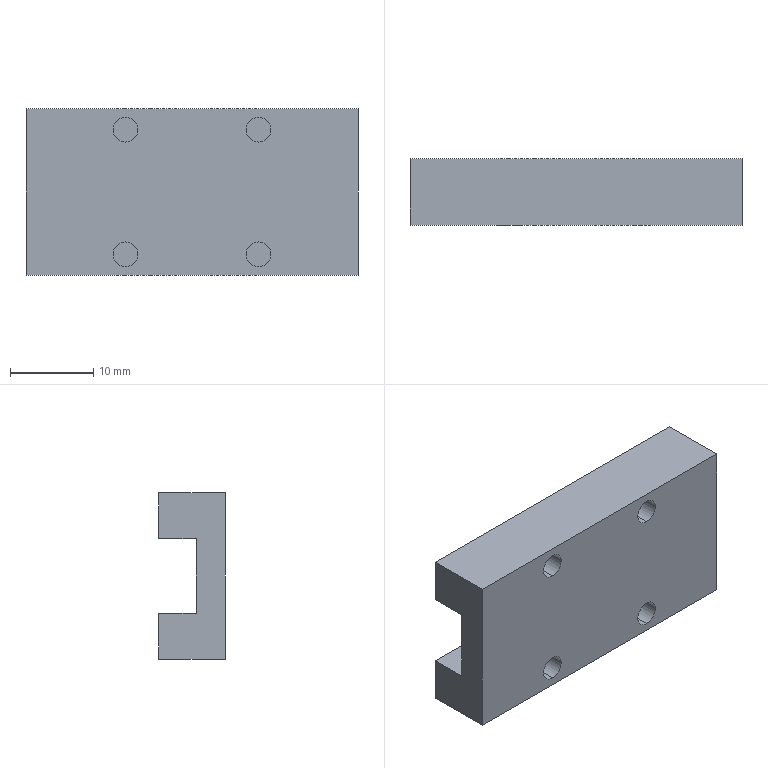Part | SolidWorks | features BaseBody 1 | 1 solid | 22 faces | box 39.9 x 8 x 20 mm | volume 4655 mm3 | plane 14 | cylinder 8 | commonest cylinder face diameters 3 x8
STEP:
#1=CARTESIAN_POINT('',(-8.,4.,9.));
#2=VERTEX_POINT('',#1);
#3=CARTESIAN_POINT('',(-8.,4.,6.));
#4=VERTEX_POINT('',#3);
#5=CARTESIAN_POINT('',(-8.,4.,7.5));
#6=DIRECTION('',(0.,-1.,0.));
#7=DIRECTION('',(0.,0.,-1.));
#8=AXIS2_PLACEMENT_3D('',#5,#6,#7);
#9=CIRCLE('',#8,1.5);
#10=EDGE_CURVE('',#2,#4,#9,.T.);
#11=ORIENTED_EDGE('',*,*,#10,.F.);
#12=CARTESIAN_POINT('',(-8.,0.,9.));
#13=VERTEX_POINT('',#12);
#14=CARTESIAN_POINT('',(-8.,4.,9.));
#15=DIRECTION('',(0.,-1.,0.));
#16=VECTOR('',#15,1000.);
#17=LINE('',#14,#16);
#18=EDGE_CURVE('',#2,#13,#17,.T.);
#19=ORIENTED_EDGE('',*,*,#18,.T.);
#20=CARTESIAN_POINT('',(-8.,0.,6.));
#21=VERTEX_POINT('',#20);
#22=CARTESIAN_POINT('',(-8.,0.,7.5));
#23=DIRECTION('',(0.,1.,0.));
#24=DIRECTION('',(0.,0.,-1.));
#25=AXIS2_PLACEMENT_3D('',#22,#23,#24);
#26=CIRCLE('',#25,1.5);
#27=EDGE_CURVE('',#21,#13,#26,.T.);
#28=ORIENTED_EDGE('',*,*,#27,.F.);
#29=CARTESIAN_POINT('',(-8.,4.,6.));
#30=DIRECTION('',(0.,-1.,0.));
#31=VECTOR('',#30,1000.);
#32=LINE('',#29,#31);
#33=EDGE_CURVE('',#4,#21,#32,.T.);
#34=ORIENTED_EDGE('',*,*,#33,.F.);
#35=EDGE_LOOP('',(#11,#19,#28,#34));
#36=FACE_OUTER_BOUND('',#35,.T.);
#37=CARTESIAN_POINT('',(-8.,4.,7.5));
#38=DIRECTION('',(0.,-1.,0.));
#39=DIRECTION('',(0.,0.,-1.));
#40=AXIS2_PLACEMENT_3D('',#37,#38,#39);
#41=CYLINDRICAL_SURFACE('',#40,1.5);
#42=ADVANCED_FACE('',(#36),#41,.F.);
#43=CARTESIAN_POINT('',(8.,4.,9.));
#44=VERTEX_POINT('',#43);
#45=CARTESIAN_POINT('',(8.,4.,6.));
#46=VERTEX_POINT('',#45);
#47=CARTESIAN_POINT('',(8.,4.,7.5));
#48=DIRECTION('',(0.,-1.,0.));
#49=DIRECTION('',(0.,0.,-1.));
#50=AXIS2_PLACEMENT_3D('',#47,#48,#49);
#51=CIRCLE('',#50,1.5);
#52=EDGE_CURVE('',#44,#46,#51,.T.);
#53=ORIENTED_EDGE('',*,*,#52,.F.);
#54=CARTESIAN_POINT('',(8.,0.,9.));
#55=VERTEX_POINT('',#54);
#56=CARTESIAN_POINT('',(8.,4.,9.));
#57=DIRECTION('',(0.,-1.,0.));
#58=VECTOR('',#57,1000.);
#59=LINE('',#56,#58);
#60=EDGE_CURVE('',#44,#55,#59,.T.);
#61=ORIENTED_EDGE('',*,*,#60,.T.);
#62=CARTESIAN_POINT('',(8.,0.,6.));
#63=VERTEX_POINT('',#62);
#64=CARTESIAN_POINT('',(8.,0.,7.5));
#65=DIRECTION('',(0.,1.,0.));
#66=DIRECTION('',(0.,0.,-1.));
#67=AXIS2_PLACEMENT_3D('',#64,#65,#66);
#68=CIRCLE('',#67,1.5);
#69=EDGE_CURVE('',#63,#55,#68,.T.);
#70=ORIENTED_EDGE('',*,*,#69,.F.);
#71=CARTESIAN_POINT('',(8.,4.,6.));
#72=DIRECTION('',(0.,-1.,0.));
#73=VECTOR('',#72,1000.);
#74=LINE('',#71,#73);
#75=EDGE_CURVE('',#46,#63,#74,.T.);
#76=ORIENTED_EDGE('',*,*,#75,.F.);
#77=EDGE_LOOP('',(#53,#61,#70,#76));
#78=FACE_OUTER_BOUND('',#77,.T.);
#79=CARTESIAN_POINT('',(8.,4.,7.5));
#80=DIRECTION('',(0.,-1.,0.));
#81=DIRECTION('',(0.,0.,-1.));
#82=AXIS2_PLACEMENT_3D('',#79,#80,#81);
#83=CYLINDRICAL_SURFACE('',#82,1.5);
#84=ADVANCED_FACE('',(#78),#83,.F.);
#85=CARTESIAN_POINT('',(8.,4.,-6.));
#86=VERTEX_POINT('',#85);
#87=CARTESIAN_POINT('',(8.,4.,-9.));
#88=VERTEX_POINT('',#87);
#89=CARTESIAN_POINT('',(8.,4.,-7.5));
#90=DIRECTION('',(0.,-1.,0.));
#91=DIRECTION('',(0.,0.,-1.));
#92=AXIS2_PLACEMENT_3D('',#89,#90,#91);
#93=CIRCLE('',#92,1.5);
#94=EDGE_CURVE('',#86,#88,#93,.T.);
#95=ORIENTED_EDGE('',*,*,#94,.F.);
#96=CARTESIAN_POINT('',(8.,0.,-6.));
#97=VERTEX_POINT('',#96);
#98=CARTESIAN_POINT('',(8.,4.,-6.));
#99=DIRECTION('',(0.,-1.,0.));
#100=VECTOR('',#99,1000.);
#101=LINE('',#98,#100);
#102=EDGE_CURVE('',#86,#97,#101,.T.);
#103=ORIENTED_EDGE('',*,*,#102,.T.);
#104=CARTESIAN_POINT('',(8.,0.,-9.));
#105=VERTEX_POINT('',#104);
#106=CARTESIAN_POINT('',(8.,0.,-7.5));
#107=DIRECTION('',(0.,1.,0.));
#108=DIRECTION('',(0.,0.,-1.));
#109=AXIS2_PLACEMENT_3D('',#106,#107,#108);
#110=CIRCLE('',#109,1.5);
#111=EDGE_CURVE('',#105,#97,#110,.T.);
#112=ORIENTED_EDGE('',*,*,#111,.F.);
#113=CARTESIAN_POINT('',(8.,4.,-9.));
#114=DIRECTION('',(0.,-1.,0.));
#115=VECTOR('',#114,1000.);
#116=LINE('',#113,#115);
#117=EDGE_CURVE('',#88,#105,#116,.T.);
#118=ORIENTED_EDGE('',*,*,#117,.F.);
#119=EDGE_LOOP('',(#95,#103,#112,#118));
#120=FACE_OUTER_BOUND('',#119,.T.);
#121=CARTESIAN_POINT('',(8.,4.,-7.5));
#122=DIRECTION('',(0.,-1.,0.));
#123=DIRECTION('',(0.,0.,-1.));
#124=AXIS2_PLACEMENT_3D('',#121,#122,#123);
#125=CYLINDRICAL_SURFACE('',#124,1.5);
#126=ADVANCED_FACE('',(#120),#125,.F.);
#127=CARTESIAN_POINT('',(-8.,4.,-6.));
#128=VERTEX_POINT('',#127);
#129=CARTESIAN_POINT('',(-8.,4.,-9.));
#130=VERTEX_POINT('',#129);
#131=CARTESIAN_POINT('',(-8.,4.,-7.5));
#132=DIRECTION('',(0.,-1.,0.));
#133=DIRECTION('',(0.,0.,-1.));
#134=AXIS2_PLACEMENT_3D('',#131,#132,#133);
#135=CIRCLE('',#134,1.5);
#136=EDGE_CURVE('',#128,#130,#135,.T.);
#137=ORIENTED_EDGE('',*,*,#136,.F.);
#138=CARTESIAN_POINT('',(-8.,0.,-6.));
#139=VERTEX_POINT('',#138);
#140=CARTESIAN_POINT('',(-8.,4.,-6.));
#141=DIRECTION('',(0.,-1.,0.));
#142=VECTOR('',#141,1000.);
#143=LINE('',#140,#142);
#144=EDGE_CURVE('',#128,#139,#143,.T.);
#145=ORIENTED_EDGE('',*,*,#144,.T.);
#146=CARTESIAN_POINT('',(-8.,0.,-9.));
#147=VERTEX_POINT('',#146);
#148=CARTESIAN_POINT('',(-8.,0.,-7.5));
#149=DIRECTION('',(0.,1.,0.));
#150=DIRECTION('',(0.,0.,-1.));
#151=AXIS2_PLACEMENT_3D('',#148,#149,#150);
#152=CIRCLE('',#151,1.5);
#153=EDGE_CURVE('',#147,#139,#152,.T.);
#154=ORIENTED_EDGE('',*,*,#153,.F.);
#155=CARTESIAN_POINT('',(-8.,4.,-9.));
#156=DIRECTION('',(0.,-1.,0.));
#157=VECTOR('',#156,1000.);
#158=LINE('',#155,#157);
#159=EDGE_CURVE('',#130,#147,#158,.T.);
#160=ORIENTED_EDGE('',*,*,#159,.F.);
#161=EDGE_LOOP('',(#137,#145,#154,#160));
#162=FACE_OUTER_BOUND('',#161,.T.);
#163=CARTESIAN_POINT('',(-8.,4.,-7.5));
#164=DIRECTION('',(0.,-1.,0.));
#165=DIRECTION('',(0.,0.,-1.));
#166=AXIS2_PLACEMENT_3D('',#163,#164,#165);
#167=CYLINDRICAL_SURFACE('',#166,1.5);
#168=ADVANCED_FACE('',(#162),#167,.F.);
#169=CARTESIAN_POINT('',(-19.95,0.,-10.));
#170=VERTEX_POINT('',#169);
#171=CARTESIAN_POINT('',(19.95,0.,-10.));
#172=VERTEX_POINT('',#171);
#173=CARTESIAN_POINT('',(0.,0.,-10.));
#174=DIRECTION('',(1.,0.,0.));
#175=VECTOR('',#174,1000.);
#176=LINE('',#173,#175);
#177=EDGE_CURVE('',#170,#172,#176,.T.);
#178=ORIENTED_EDGE('',*,*,#177,.T.);
#179=CARTESIAN_POINT('',(19.95,0.,10.));
#180=VERTEX_POINT('',#179);
#181=CARTESIAN_POINT('',(19.95,0.,0.));
#182=DIRECTION('',(0.,0.,1.));
#183=VECTOR('',#182,1000.);
#184=LINE('',#181,#183);
#185=EDGE_CURVE('',#172,#180,#184,.T.);
#186=ORIENTED_EDGE('',*,*,#185,.T.);
#187=CARTESIAN_POINT('',(-19.95,0.,10.));
#188=VERTEX_POINT('',#187);
#189=CARTESIAN_POINT('',(0.,0.,10.));
#190=DIRECTION('',(-1.,0.,0.));
#191=VECTOR('',#190,1000.);
#192=LINE('',#189,#191);
#193=EDGE_CURVE('',#180,#188,#192,.T.);
#194=ORIENTED_EDGE('',*,*,#193,.T.);
#195=CARTESIAN_POINT('',(-19.95,0.,0.));
#196=DIRECTION('',(0.,0.,-1.));
#197=VECTOR('',#196,1000.);
#198=LINE('',#195,#197);
#199=EDGE_CURVE('',#188,#170,#198,.T.);
#200=ORIENTED_EDGE('',*,*,#199,.T.);
#201=EDGE_LOOP('',(#178,#186,#194,#200));
#202=FACE_OUTER_BOUND('',#201,.T.);
#203=ORIENTED_EDGE('',*,*,#27,.T.);
#204=CARTESIAN_POINT('',(-8.,0.,7.5));
#205=DIRECTION('',(0.,1.,0.));
#206=DIRECTION('',(0.,0.,-1.));
#207=AXIS2_PLACEMENT_3D('',#204,#205,#206);
#208=CIRCLE('',#207,1.5);
#209=EDGE_CURVE('',#13,#21,#208,.T.);
#210=ORIENTED_EDGE('',*,*,#209,.T.);
#211=EDGE_LOOP('',(#203,#210));
#212=FACE_BOUND('',#211,.T.);
#213=ORIENTED_EDGE('',*,*,#69,.T.);
#214=CARTESIAN_POINT('',(8.,0.,7.5));
#215=DIRECTION('',(0.,1.,0.));
#216=DIRECTION('',(0.,0.,-1.));
#217=AXIS2_PLACEMENT_3D('',#214,#215,#216);
#218=CIRCLE('',#217,1.5);
#219=EDGE_CURVE('',#55,#63,#218,.T.);
#220=ORIENTED_EDGE('',*,*,#219,.T.);
#221=EDGE_LOOP('',(#213,#220));
#222=FACE_BOUND('',#221,.T.);
#223=ORIENTED_EDGE('',*,*,#111,.T.);
#224=CARTESIAN_POINT('',(8.,0.,-7.5));
#225=DIRECTION('',(0.,1.,0.));
#226=DIRECTION('',(0.,0.,-1.));
#227=AXIS2_PLACEMENT_3D('',#224,#225,#226);
#228=CIRCLE('',#227,1.5);
#229=EDGE_CURVE('',#97,#105,#228,.T.);
#230=ORIENTED_EDGE('',*,*,#229,.T.);
#231=EDGE_LOOP('',(#223,#230));
#232=FACE_BOUND('',#231,.T.);
#233=ORIENTED_EDGE('',*,*,#153,.T.);
#234=CARTESIAN_POINT('',(-8.,0.,-7.5));
#235=DIRECTION('',(0.,1.,0.));
#236=DIRECTION('',(0.,0.,-1.));
#237=AXIS2_PLACEMENT_3D('',#234,#235,#236);
#238=CIRCLE('',#237,1.5);
#239=EDGE_CURVE('',#139,#147,#238,.T.);
#240=ORIENTED_EDGE('',*,*,#239,.T.);
#241=EDGE_LOOP('',(#233,#240));
#242=FACE_BOUND('',#241,.T.);
#243=CARTESIAN_POINT('',(0.,0.,0.));
#244=DIRECTION('',(0.,-1.,0.));
#245=DIRECTION('',(0.,0.,-1.));
#246=AXIS2_PLACEMENT_3D('',#243,#244,#245);
#247=PLANE('',#246);
#248=ADVANCED_FACE('',(#202,#212,#222,#232,#242),#247,.T.);
#249=CARTESIAN_POINT('',(19.95,8.,-10.));
#250=VERTEX_POINT('',#249);
#251=CARTESIAN_POINT('',(-19.95,8.,-10.));
#252=VERTEX_POINT('',#251);
#253=CARTESIAN_POINT('',(-19.95,8.,-10.));
#254=DIRECTION('',(-1.,0.,0.));
#255=VECTOR('',#254,1000.);
#256=LINE('',#253,#255);
#257=EDGE_CURVE('',#250,#252,#256,.T.);
#258=ORIENTED_EDGE('',*,*,#257,.F.);
#259=CARTESIAN_POINT('',(19.95,8.,-10.));
#260=DIRECTION('',(0.,-1.,0.));
#261=VECTOR('',#260,1000.);
#262=LINE('',#259,#261);
#263=EDGE_CURVE('',#250,#172,#262,.T.);
#264=ORIENTED_EDGE('',*,*,#263,.T.);
#265=ORIENTED_EDGE('',*,*,#177,.F.);
#266=CARTESIAN_POINT('',(-19.95,8.,-10.));
#267=DIRECTION('',(0.,-1.,0.));
#268=VECTOR('',#267,1000.);
#269=LINE('',#266,#268);
#270=EDGE_CURVE('',#252,#170,#269,.T.);
#271=ORIENTED_EDGE('',*,*,#270,.F.);
#272=EDGE_LOOP('',(#258,#264,#265,#271));
#273=FACE_OUTER_BOUND('',#272,.T.);
#274=CARTESIAN_POINT('',(-19.95,8.,-10.));
#275=DIRECTION('',(0.,0.,1.));
#276=DIRECTION('',(1.,0.,0.));
#277=AXIS2_PLACEMENT_3D('',#274,#275,#276);
#278=PLANE('',#277);
#279=ADVANCED_FACE('',(#273),#278,.F.);
#280=ORIENTED_EDGE('',*,*,#193,.F.);
#281=CARTESIAN_POINT('',(19.95,8.,10.));
#282=VERTEX_POINT('',#281);
#283=CARTESIAN_POINT('',(19.95,8.,10.));
#284=DIRECTION('',(0.,1.,0.));
#285=VECTOR('',#284,1000.);
#286=LINE('',#283,#285);
#287=EDGE_CURVE('',#180,#282,#286,.T.);
#288=ORIENTED_EDGE('',*,*,#287,.T.);
#289=CARTESIAN_POINT('',(-19.95,8.,10.));
#290=VERTEX_POINT('',#289);
#291=CARTESIAN_POINT('',(-19.95,8.,10.));
#292=DIRECTION('',(1.,0.,0.));
#293=VECTOR('',#292,1000.);
#294=LINE('',#291,#293);
#295=EDGE_CURVE('',#290,#282,#294,.T.);
#296=ORIENTED_EDGE('',*,*,#295,.F.);
#297=CARTESIAN_POINT('',(-19.95,8.,10.));
#298=DIRECTION('',(0.,-1.,0.));
#299=VECTOR('',#298,1000.);
#300=LINE('',#297,#299);
#301=EDGE_CURVE('',#290,#188,#300,.T.);
#302=ORIENTED_EDGE('',*,*,#301,.T.);
#303=EDGE_LOOP('',(#280,#288,#296,#302));
#304=FACE_OUTER_BOUND('',#303,.T.);
#305=CARTESIAN_POINT('',(-19.95,8.,10.));
#306=DIRECTION('',(0.,0.,-1.));
#307=DIRECTION('',(-1.,0.,0.));
#308=AXIS2_PLACEMENT_3D('',#305,#306,#307);
#309=PLANE('',#308);
#310=ADVANCED_FACE('',(#304),#309,.F.);
#311=ORIENTED_EDGE('',*,*,#18,.F.);
#312=CARTESIAN_POINT('',(-8.,4.,7.5));
#313=DIRECTION('',(0.,-1.,0.));
#314=DIRECTION('',(0.,0.,-1.));
#315=AXIS2_PLACEMENT_3D('',#312,#313,#314);
#316=CIRCLE('',#315,1.5);
#317=EDGE_CURVE('',#4,#2,#316,.T.);
#318=ORIENTED_EDGE('',*,*,#317,.F.);
#319=ORIENTED_EDGE('',*,*,#33,.T.);
#320=ORIENTED_EDGE('',*,*,#209,.F.);
#321=EDGE_LOOP('',(#311,#318,#319,#320));
#322=FACE_OUTER_BOUND('',#321,.T.);
#323=CARTESIAN_POINT('',(-8.,4.,7.5));
#324=DIRECTION('',(0.,-1.,0.));
#325=DIRECTION('',(0.,0.,-1.));
#326=AXIS2_PLACEMENT_3D('',#323,#324,#325);
#327=CYLINDRICAL_SURFACE('',#326,1.5);
#328=ADVANCED_FACE('',(#322),#327,.F.);
#329=ORIENTED_EDGE('',*,*,#60,.F.);
#330=CARTESIAN_POINT('',(8.,4.,7.5));
#331=DIRECTION('',(0.,-1.,0.));
#332=DIRECTION('',(0.,0.,-1.));
#333=AXIS2_PLACEMENT_3D('',#330,#331,#332);
#334=CIRCLE('',#333,1.5);
#335=EDGE_CURVE('',#46,#44,#334,.T.);
#336=ORIENTED_EDGE('',*,*,#335,.F.);
#337=ORIENTED_EDGE('',*,*,#75,.T.);
#338=ORIENTED_EDGE('',*,*,#219,.F.);
#339=EDGE_LOOP('',(#329,#336,#337,#338));
#340=FACE_OUTER_BOUND('',#339,.T.);
#341=CARTESIAN_POINT('',(8.,4.,7.5));
#342=DIRECTION('',(0.,-1.,0.));
#343=DIRECTION('',(0.,0.,-1.));
#344=AXIS2_PLACEMENT_3D('',#341,#342,#343);
#345=CYLINDRICAL_SURFACE('',#344,1.5);
#346=ADVANCED_FACE('',(#340),#345,.F.);
#347=ORIENTED_EDGE('',*,*,#102,.F.);
#348=CARTESIAN_POINT('',(8.,4.,-7.5));
#349=DIRECTION('',(0.,-1.,0.));
#350=DIRECTION('',(0.,0.,-1.));
#351=AXIS2_PLACEMENT_3D('',#348,#349,#350);
#352=CIRCLE('',#351,1.5);
#353=EDGE_CURVE('',#88,#86,#352,.T.);
#354=ORIENTED_EDGE('',*,*,#353,.F.);
#355=ORIENTED_EDGE('',*,*,#117,.T.);
#356=ORIENTED_EDGE('',*,*,#229,.F.);
#357=EDGE_LOOP('',(#347,#354,#355,#356));
#358=FACE_OUTER_BOUND('',#357,.T.);
#359=CARTESIAN_POINT('',(8.,4.,-7.5));
#360=DIRECTION('',(0.,-1.,0.));
#361=DIRECTION('',(0.,0.,-1.));
#362=AXIS2_PLACEMENT_3D('',#359,#360,#361);
#363=CYLINDRICAL_SURFACE('',#362,1.5);
#364=ADVANCED_FACE('',(#358),#363,.F.);
#365=ORIENTED_EDGE('',*,*,#144,.F.);
#366=CARTESIAN_POINT('',(-8.,4.,-7.5));
#367=DIRECTION('',(0.,-1.,0.));
#368=DIRECTION('',(0.,0.,-1.));
#369=AXIS2_PLACEMENT_3D('',#366,#367,#368);
#370=CIRCLE('',#369,1.5);
#371=EDGE_CURVE('',#130,#128,#370,.T.);
#372=ORIENTED_EDGE('',*,*,#371,.F.);
#373=ORIENTED_EDGE('',*,*,#159,.T.);
#374=ORIENTED_EDGE('',*,*,#239,.F.);
#375=EDGE_LOOP('',(#365,#372,#373,#374));
#376=FACE_OUTER_BOUND('',#375,.T.);
#377=CARTESIAN_POINT('',(-8.,4.,-7.5));
#378=DIRECTION('',(0.,-1.,0.));
#379=DIRECTION('',(0.,0.,-1.));
#380=AXIS2_PLACEMENT_3D('',#377,#378,#379);
#381=CYLINDRICAL_SURFACE('',#380,1.5);
#382=ADVANCED_FACE('',(#376),#381,.F.);
#383=CARTESIAN_POINT('',(19.95,8.,-4.5));
#384=VERTEX_POINT('',#383);
#385=CARTESIAN_POINT('',(-19.95,8.,-4.5));
#386=VERTEX_POINT('',#385);
#387=CARTESIAN_POINT('',(0.,8.,-4.5));
#388=DIRECTION('',(-1.,0.,0.));
#389=VECTOR('',#388,1000.);
#390=LINE('',#387,#389);
#391=EDGE_CURVE('',#384,#386,#390,.T.);
#392=ORIENTED_EDGE('',*,*,#391,.F.);
#393=CARTESIAN_POINT('',(19.95,8.,0.));
#394=DIRECTION('',(0.,0.,1.));
#395=VECTOR('',#394,1000.);
#396=LINE('',#393,#395);
#397=EDGE_CURVE('',#250,#384,#396,.T.);
#398=ORIENTED_EDGE('',*,*,#397,.F.);
#399=ORIENTED_EDGE('',*,*,#257,.T.);
#400=CARTESIAN_POINT('',(-19.95,8.,0.));
#401=DIRECTION('',(0.,0.,-1.));
#402=VECTOR('',#401,1000.);
#403=LINE('',#400,#402);
#404=EDGE_CURVE('',#386,#252,#403,.T.);
#405=ORIENTED_EDGE('',*,*,#404,.F.);
#406=EDGE_LOOP('',(#392,#398,#399,#405));
#407=FACE_OUTER_BOUND('',#406,.T.);
#408=CARTESIAN_POINT('',(0.,8.,0.));
#409=DIRECTION('',(0.,-1.,0.));
#410=DIRECTION('',(0.,0.,-1.));
#411=AXIS2_PLACEMENT_3D('',#408,#409,#410);
#412=PLANE('',#411);
#413=ADVANCED_FACE('',(#407),#412,.F.);
#414=CARTESIAN_POINT('',(-19.95,8.,4.5));
#415=VERTEX_POINT('',#414);
#416=CARTESIAN_POINT('',(19.95,8.,4.5));
#417=VERTEX_POINT('',#416);
#418=CARTESIAN_POINT('',(0.,8.,4.5));
#419=DIRECTION('',(1.,0.,0.));
#420=VECTOR('',#419,1000.);
#421=LINE('',#418,#420);
#422=EDGE_CURVE('',#415,#417,#421,.T.);
#423=ORIENTED_EDGE('',*,*,#422,.F.);
#424=CARTESIAN_POINT('',(-19.95,8.,0.));
#425=DIRECTION('',(0.,0.,-1.));
#426=VECTOR('',#425,1000.);
#427=LINE('',#424,#426);
#428=EDGE_CURVE('',#290,#415,#427,.T.);
#429=ORIENTED_EDGE('',*,*,#428,.F.);
#430=ORIENTED_EDGE('',*,*,#295,.T.);
#431=CARTESIAN_POINT('',(19.95,8.,0.));
#432=DIRECTION('',(0.,0.,1.));
#433=VECTOR('',#432,1000.);
#434=LINE('',#431,#433);
#435=EDGE_CURVE('',#417,#282,#434,.T.);
#436=ORIENTED_EDGE('',*,*,#435,.F.);
#437=EDGE_LOOP('',(#423,#429,#430,#436));
#438=FACE_OUTER_BOUND('',#437,.T.);
#439=CARTESIAN_POINT('',(0.,8.,0.));
#440=DIRECTION('',(0.,-1.,0.));
#441=DIRECTION('',(0.,0.,-1.));
#442=AXIS2_PLACEMENT_3D('',#439,#440,#441);
#443=PLANE('',#442);
#444=ADVANCED_FACE('',(#438),#443,.F.);
#445=ORIENTED_EDGE('',*,*,#317,.T.);
#446=ORIENTED_EDGE('',*,*,#10,.T.);
#447=EDGE_LOOP('',(#445,#446));
#448=FACE_OUTER_BOUND('',#447,.T.);
#449=CARTESIAN_POINT('',(-8.,4.,7.5));
#450=DIRECTION('',(0.,-1.,0.));
#451=DIRECTION('',(0.,0.,-1.));
#452=AXIS2_PLACEMENT_3D('',#449,#450,#451);
#453=PLANE('',#452);
#454=ADVANCED_FACE('',(#448),#453,.T.);
#455=ORIENTED_EDGE('',*,*,#335,.T.);
#456=ORIENTED_EDGE('',*,*,#52,.T.);
#457=EDGE_LOOP('',(#455,#456));
#458=FACE_OUTER_BOUND('',#457,.T.);
#459=CARTESIAN_POINT('',(8.,4.,7.5));
#460=DIRECTION('',(0.,1.,0.));
#461=DIRECTION('',(0.,0.,1.));
#462=AXIS2_PLACEMENT_3D('',#459,#460,#461);
#463=PLANE('',#462);
#464=ADVANCED_FACE('',(#458),#463,.F.);
#465=ORIENTED_EDGE('',*,*,#353,.T.);
#466=ORIENTED_EDGE('',*,*,#94,.T.);
#467=EDGE_LOOP('',(#465,#466));
#468=FACE_OUTER_BOUND('',#467,.T.);
#469=CARTESIAN_POINT('',(8.,4.,-7.5));
#470=DIRECTION('',(0.,-1.,0.));
#471=DIRECTION('',(0.,0.,-1.));
#472=AXIS2_PLACEMENT_3D('',#469,#470,#471);
#473=PLANE('',#472);
#474=ADVANCED_FACE('',(#468),#473,.T.);
#475=ORIENTED_EDGE('',*,*,#371,.T.);
#476=ORIENTED_EDGE('',*,*,#136,.T.);
#477=EDGE_LOOP('',(#475,#476));
#478=FACE_OUTER_BOUND('',#477,.T.);
#479=CARTESIAN_POINT('',(-8.,4.,-7.5));
#480=DIRECTION('',(0.,1.,0.));
#481=DIRECTION('',(0.,0.,1.));
#482=AXIS2_PLACEMENT_3D('',#479,#480,#481);
#483=PLANE('',#482);
#484=ADVANCED_FACE('',(#478),#483,.F.);
#485=CARTESIAN_POINT('',(19.95,3.5,4.5));
#486=VERTEX_POINT('',#485);
#487=CARTESIAN_POINT('',(19.95,8.,4.5));
#488=DIRECTION('',(0.,-1.,0.));
#489=VECTOR('',#488,1000.);
#490=LINE('',#487,#489);
#491=EDGE_CURVE('',#417,#486,#490,.T.);
#492=ORIENTED_EDGE('',*,*,#491,.F.);
#493=ORIENTED_EDGE('',*,*,#435,.T.);
#494=ORIENTED_EDGE('',*,*,#287,.F.);
#495=ORIENTED_EDGE('',*,*,#185,.F.);
#496=ORIENTED_EDGE('',*,*,#263,.F.);
#497=ORIENTED_EDGE('',*,*,#397,.T.);
#498=CARTESIAN_POINT('',(19.95,3.5,-4.5));
#499=VERTEX_POINT('',#498);
#500=CARTESIAN_POINT('',(19.95,8.,-4.5));
#501=DIRECTION('',(0.,1.,0.));
#502=VECTOR('',#501,1000.);
#503=LINE('',#500,#502);
#504=EDGE_CURVE('',#499,#384,#503,.T.);
#505=ORIENTED_EDGE('',*,*,#504,.F.);
#506=CARTESIAN_POINT('',(19.95,3.5,10.));
#507=DIRECTION('',(0.,0.,-1.));
#508=VECTOR('',#507,1000.);
#509=LINE('',#506,#508);
#510=EDGE_CURVE('',#486,#499,#509,.T.);
#511=ORIENTED_EDGE('',*,*,#510,.F.);
#512=EDGE_LOOP('',(#492,#493,#494,#495,#496,#497,#505,#511));
#513=FACE_OUTER_BOUND('',#512,.T.);
#514=CARTESIAN_POINT('',(19.95,8.,10.));
#515=DIRECTION('',(-1.,0.,0.));
#516=DIRECTION('',(0.,0.,1.));
#517=AXIS2_PLACEMENT_3D('',#514,#515,#516);
#518=PLANE('',#517);
#519=ADVANCED_FACE('',(#513),#518,.F.);
#520=CARTESIAN_POINT('',(-19.95,3.5,4.5));
#521=VERTEX_POINT('',#520);
#522=CARTESIAN_POINT('',(-19.95,8.,4.5));
#523=DIRECTION('',(0.,1.,0.));
#524=VECTOR('',#523,1000.);
#525=LINE('',#522,#524);
#526=EDGE_CURVE('',#521,#415,#525,.T.);
#527=ORIENTED_EDGE('',*,*,#526,.F.);
#528=CARTESIAN_POINT('',(-19.95,3.5,-4.5));
#529=VERTEX_POINT('',#528);
#530=CARTESIAN_POINT('',(-19.95,3.5,10.));
#531=DIRECTION('',(0.,0.,1.));
#532=VECTOR('',#531,1000.);
#533=LINE('',#530,#532);
#534=EDGE_CURVE('',#529,#521,#533,.T.);
#535=ORIENTED_EDGE('',*,*,#534,.F.);
#536=CARTESIAN_POINT('',(-19.95,8.,-4.5));
#537=DIRECTION('',(0.,-1.,0.));
#538=VECTOR('',#537,1000.);
#539=LINE('',#536,#538);
#540=EDGE_CURVE('',#386,#529,#539,.T.);
#541=ORIENTED_EDGE('',*,*,#540,.F.);
#542=ORIENTED_EDGE('',*,*,#404,.T.);
#543=ORIENTED_EDGE('',*,*,#270,.T.);
#544=ORIENTED_EDGE('',*,*,#199,.F.);
#545=ORIENTED_EDGE('',*,*,#301,.F.);
#546=ORIENTED_EDGE('',*,*,#428,.T.);
#547=EDGE_LOOP('',(#527,#535,#541,#542,#543,#544,#545,#546));
#548=FACE_OUTER_BOUND('',#547,.T.);
#549=CARTESIAN_POINT('',(-19.95,8.,10.));
#550=DIRECTION('',(1.,0.,0.));
#551=DIRECTION('',(0.,0.,-1.));
#552=AXIS2_PLACEMENT_3D('',#549,#550,#551);
#553=PLANE('',#552);
#554=ADVANCED_FACE('',(#548),#553,.F.);
#555=ORIENTED_EDGE('',*,*,#540,.T.);
#556=CARTESIAN_POINT('',(-19.95,3.5,-4.5));
#557=DIRECTION('',(-1.,0.,0.));
#558=VECTOR('',#557,1000.);
#559=LINE('',#556,#558);
#560=EDGE_CURVE('',#499,#529,#559,.T.);
#561=ORIENTED_EDGE('',*,*,#560,.F.);
#562=ORIENTED_EDGE('',*,*,#504,.T.);
#563=ORIENTED_EDGE('',*,*,#391,.T.);
#564=EDGE_LOOP('',(#555,#561,#562,#563));
#565=FACE_OUTER_BOUND('',#564,.T.);
#566=CARTESIAN_POINT('',(-19.95,3.5,-4.5));
#567=DIRECTION('',(0.,0.,-1.));
#568=DIRECTION('',(-1.,0.,0.));
#569=AXIS2_PLACEMENT_3D('',#566,#567,#568);
#570=PLANE('',#569);
#571=ADVANCED_FACE('',(#565),#570,.F.);
#572=ORIENTED_EDGE('',*,*,#491,.T.);
#573=CARTESIAN_POINT('',(-19.95,3.5,4.5));
#574=DIRECTION('',(1.,0.,0.));
#575=VECTOR('',#574,1000.);
#576=LINE('',#573,#575);
#577=EDGE_CURVE('',#521,#486,#576,.T.);
#578=ORIENTED_EDGE('',*,*,#577,.F.);
#579=ORIENTED_EDGE('',*,*,#526,.T.);
#580=ORIENTED_EDGE('',*,*,#422,.T.);
#581=EDGE_LOOP('',(#572,#578,#579,#580));
#582=FACE_OUTER_BOUND('',#581,.T.);
#583=CARTESIAN_POINT('',(-19.95,3.5,4.5));
#584=DIRECTION('',(0.,0.,1.));
#585=DIRECTION('',(1.,0.,0.));
#586=AXIS2_PLACEMENT_3D('',#583,#584,#585);
#587=PLANE('',#586);
#588=ADVANCED_FACE('',(#582),#587,.F.);
#589=ORIENTED_EDGE('',*,*,#560,.T.);
#590=ORIENTED_EDGE('',*,*,#534,.T.);
#591=ORIENTED_EDGE('',*,*,#577,.T.);
#592=ORIENTED_EDGE('',*,*,#510,.T.);
#593=EDGE_LOOP('',(#589,#590,#591,#592));
#594=FACE_OUTER_BOUND('',#593,.T.);
#595=CARTESIAN_POINT('',(0.,3.5,0.));
#596=DIRECTION('',(0.,-1.,0.));
#597=DIRECTION('',(0.,0.,-1.));
#598=AXIS2_PLACEMENT_3D('',#595,#596,#597);
#599=PLANE('',#598);
#600=ADVANCED_FACE('',(#594),#599,.F.);
#601=CLOSED_SHELL('',(#42,#84,#126,#168,#248,#279,#310,#328,#346,#364,#382,#413,#444,#454,#464,#474,#484,#519,#554,#571,#588,#600));
#602=MANIFOLD_SOLID_BREP('',#601);
#603=CARTESIAN_POINT('',(0.,0.,0.));
#604=DIRECTION('',(0.,0.,1.));
#605=DIRECTION('',(1.,0.,0.));
#606=AXIS2_PLACEMENT_3D('',#603,#604,#605);
#607=(LENGTH_UNIT()NAMED_UNIT(*)SI_UNIT(.MILLI.,.METRE.));
#608=UNCERTAINTY_MEASURE_WITH_UNIT(LENGTH_MEASURE(0.00001),#607,'','');
#609=(NAMED_UNIT(*)PLANE_ANGLE_UNIT()SI_UNIT($,.RADIAN.));
#610=(NAMED_UNIT(*)SI_UNIT($,.STERADIAN.)SOLID_ANGLE_UNIT());
#611=(GEOMETRIC_REPRESENTATION_CONTEXT(3)GLOBAL_UNCERTAINTY_ASSIGNED_CONTEXT((#608))GLOBAL_UNIT_ASSIGNED_CONTEXT((#607,#609,#610))REPRESENTATION_CONTEXT('',''));
#612=ADVANCED_BREP_SHAPE_REPRESENTATION('',(#602,#606),#611);